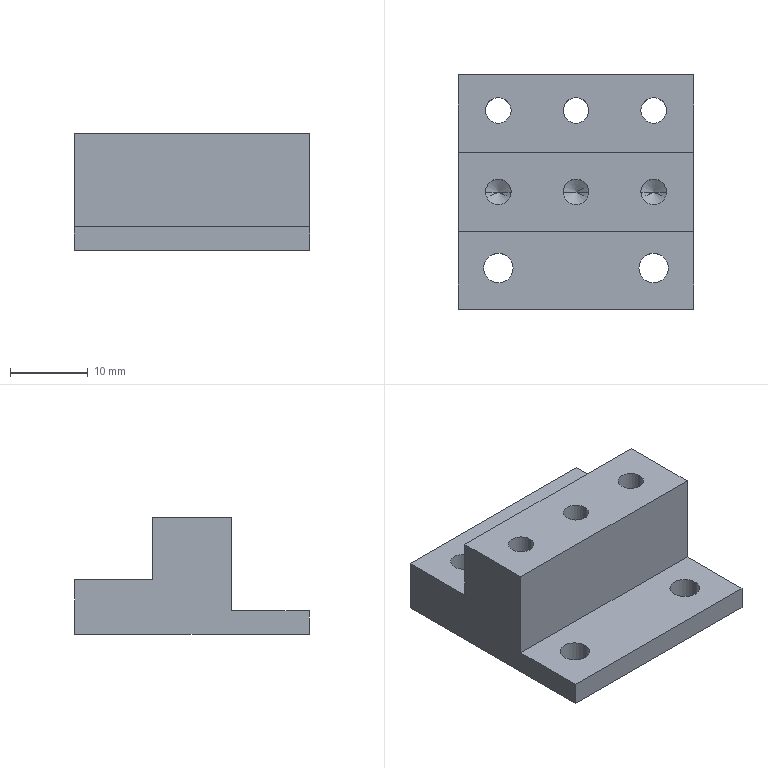Part | STEP file | Six-position grounding copper block | 1 solid | 32 faces | box 30.3 x 30.2 x 15 mm | volume 7115 mm3 | cylinder 16 | plane 10 | cone 6 | commonest cylinder face diameters 3.3 x12 3.8 x4